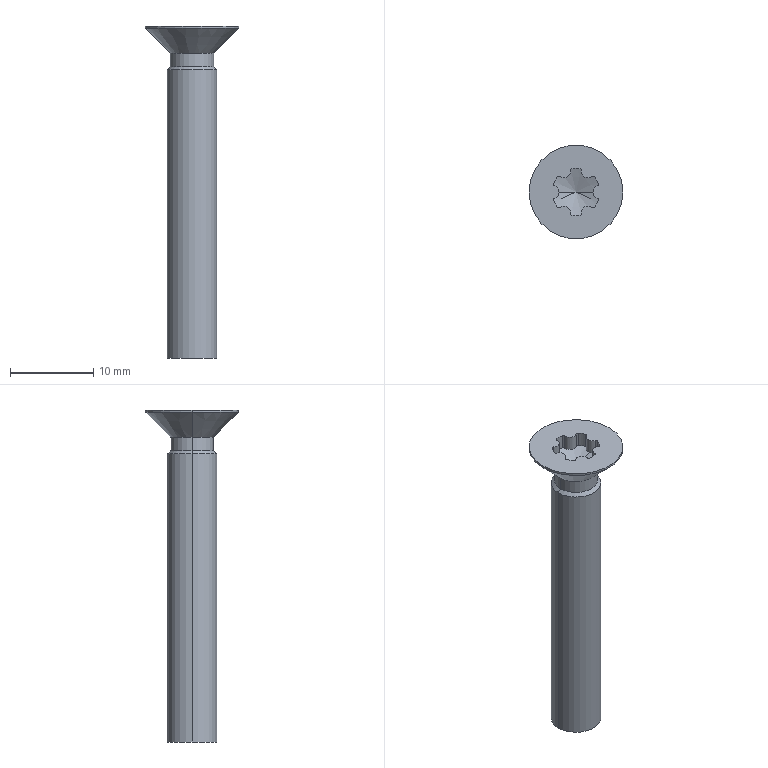Part | SolidWorks | features RevCut 2, Cut 1, Extrusion 1, LPattern 1, Revolution 1 | 1 solid | 51 faces | box 11.3 x 11.3 x 40 mm | volume 1175 mm3 | cylinder 37 | plane 8 | cone 6 | commonest cylinder face diameters 0.4 x16 1.57 x9 5.72 x6 5.196 x2 6 x2 11.3 x2
STEP:
#1=CARTESIAN_POINT('',(0.,0.,37.159));
#2=VERTEX_POINT('',#1);
#3=CARTESIAN_POINT('',(2.86,0.,38.2));
#4=VERTEX_POINT('',#3);
#5=CARTESIAN_POINT('',(2.86,0.,38.2));
#6=DIRECTION('',(0.9397,0.,0.342));
#7=VECTOR('',#6,1000.);
#8=LINE('',#5,#7);
#9=EDGE_CURVE('',#2,#4,#8,.T.);
#10=ORIENTED_EDGE('',*,*,#9,.F.);
#11=CARTESIAN_POINT('',(-2.86,0.,38.2));
#12=VERTEX_POINT('',#11);
#13=CARTESIAN_POINT('',(-2.86,0.,38.2));
#14=DIRECTION('',(-0.9397,0.,0.342));
#15=VECTOR('',#14,1000.);
#16=LINE('',#13,#15);
#17=EDGE_CURVE('',#2,#12,#16,.T.);
#18=ORIENTED_EDGE('',*,*,#17,.T.);
#19=CARTESIAN_POINT('',(-2.685,-0.9847,38.2));
#20=VERTEX_POINT('',#19);
#21=CARTESIAN_POINT('',(0.,0.,38.2));
#22=DIRECTION('',(0.,0.,-1.));
#23=DIRECTION('',(-1.,0.,0.));
#24=AXIS2_PLACEMENT_3D('',#21,#22,#23);
#25=CIRCLE('',#24,2.86);
#26=EDGE_CURVE('',#20,#12,#25,.T.);
#27=ORIENTED_EDGE('',*,*,#26,.F.);
#28=CARTESIAN_POINT('',(-2.195,-1.833,38.2));
#29=VERTEX_POINT('',#28);
#30=CARTESIAN_POINT('',(0.,0.,38.2));
#31=DIRECTION('',(0.,0.,1.));
#32=DIRECTION('',(1.,0.,0.));
#33=AXIS2_PLACEMENT_3D('',#30,#31,#32);
#34=CIRCLE('',#33,2.86);
#35=EDGE_CURVE('',#20,#29,#34,.T.);
#36=ORIENTED_EDGE('',*,*,#35,.T.);
#37=CARTESIAN_POINT('',(-0.4898,-2.818,38.2));
#38=VERTEX_POINT('',#37);
#39=CARTESIAN_POINT('',(0.,0.,38.2));
#40=DIRECTION('',(0.,0.,-1.));
#41=DIRECTION('',(-1.,0.,0.));
#42=AXIS2_PLACEMENT_3D('',#39,#40,#41);
#43=CIRCLE('',#42,2.86);
#44=EDGE_CURVE('',#38,#29,#43,.T.);
#45=ORIENTED_EDGE('',*,*,#44,.F.);
#46=CARTESIAN_POINT('',(0.4898,-2.818,38.2));
#47=VERTEX_POINT('',#46);
#48=CARTESIAN_POINT('',(0.,0.,38.2));
#49=DIRECTION('',(0.,0.,1.));
#50=DIRECTION('',(1.,0.,0.));
#51=AXIS2_PLACEMENT_3D('',#48,#49,#50);
#52=CIRCLE('',#51,2.86);
#53=EDGE_CURVE('',#38,#47,#52,.T.);
#54=ORIENTED_EDGE('',*,*,#53,.T.);
#55=CARTESIAN_POINT('',(2.195,-1.833,38.2));
#56=VERTEX_POINT('',#55);
#57=CARTESIAN_POINT('',(0.,0.,38.2));
#58=DIRECTION('',(0.,0.,-1.));
#59=DIRECTION('',(-1.,0.,0.));
#60=AXIS2_PLACEMENT_3D('',#57,#58,#59);
#61=CIRCLE('',#60,2.86);
#62=EDGE_CURVE('',#56,#47,#61,.T.);
#63=ORIENTED_EDGE('',*,*,#62,.F.);
#64=CARTESIAN_POINT('',(2.685,-0.9847,38.2));
#65=VERTEX_POINT('',#64);
#66=CARTESIAN_POINT('',(0.,0.,38.2));
#67=DIRECTION('',(0.,0.,1.));
#68=DIRECTION('',(1.,0.,0.));
#69=AXIS2_PLACEMENT_3D('',#66,#67,#68);
#70=CIRCLE('',#69,2.86);
#71=EDGE_CURVE('',#56,#65,#70,.T.);
#72=ORIENTED_EDGE('',*,*,#71,.T.);
#73=CARTESIAN_POINT('',(0.,0.,38.2));
#74=DIRECTION('',(0.,0.,-1.));
#75=DIRECTION('',(-1.,0.,0.));
#76=AXIS2_PLACEMENT_3D('',#73,#74,#75);
#77=CIRCLE('',#76,2.86);
#78=EDGE_CURVE('',#4,#65,#77,.T.);
#79=ORIENTED_EDGE('',*,*,#78,.F.);
#80=EDGE_LOOP('',(#10,#18,#27,#36,#45,#54,#63,#72,#79));
#81=FACE_OUTER_BOUND('',#80,.T.);
#82=CARTESIAN_POINT('',(0.,0.,38.2));
#83=DIRECTION('',(0.,0.,1.));
#84=DIRECTION('',(1.,0.,0.));
#85=AXIS2_PLACEMENT_3D('',#82,#83,#84);
#86=CONICAL_SURFACE('',#85,2.86,1.222);
#87=ADVANCED_FACE('',(#81),#86,.F.);
#88=CARTESIAN_POINT('',(-1.918,1.862,38.2));
#89=VERTEX_POINT('',#88);
#90=CARTESIAN_POINT('',(-0.645,2.477,38.2));
#91=VERTEX_POINT('',#90);
#92=CARTESIAN_POINT('',(-1.43,2.477,38.2));
#93=DIRECTION('',(0.,0.,1.));
#94=DIRECTION('',(1.,0.,0.));
#95=AXIS2_PLACEMENT_3D('',#92,#93,#94);
#96=CIRCLE('',#95,0.785);
#97=EDGE_CURVE('',#89,#91,#96,.T.);
#98=ORIENTED_EDGE('',*,*,#97,.T.);
#99=CARTESIAN_POINT('',(-0.645,2.477,40.));
#100=VERTEX_POINT('',#99);
#101=CARTESIAN_POINT('',(-0.645,2.477,38.2));
#102=DIRECTION('',(0.,0.,1.));
#103=VECTOR('',#102,1000.);
#104=LINE('',#101,#103);
#105=EDGE_CURVE('',#91,#100,#104,.T.);
#106=ORIENTED_EDGE('',*,*,#105,.T.);
#107=CARTESIAN_POINT('',(-1.918,1.862,40.));
#108=VERTEX_POINT('',#107);
#109=CARTESIAN_POINT('',(-1.43,2.477,40.));
#110=DIRECTION('',(0.,0.,1.));
#111=DIRECTION('',(1.,0.,0.));
#112=AXIS2_PLACEMENT_3D('',#109,#110,#111);
#113=CIRCLE('',#112,0.785);
#114=EDGE_CURVE('',#108,#100,#113,.T.);
#115=ORIENTED_EDGE('',*,*,#114,.F.);
#116=CARTESIAN_POINT('',(-1.918,1.862,38.2));
#117=DIRECTION('',(0.,0.,1.));
#118=VECTOR('',#117,1000.);
#119=LINE('',#116,#118);
#120=EDGE_CURVE('',#89,#108,#119,.T.);
#121=ORIENTED_EDGE('',*,*,#120,.F.);
#122=EDGE_LOOP('',(#98,#106,#115,#121));
#123=FACE_OUTER_BOUND('',#122,.T.);
#124=CARTESIAN_POINT('',(-1.43,2.477,38.2));
#125=DIRECTION('',(0.,0.,1.));
#126=DIRECTION('',(1.,0.,0.));
#127=AXIS2_PLACEMENT_3D('',#124,#125,#126);
#128=CYLINDRICAL_SURFACE('',#127,0.785);
#129=ADVANCED_FACE('',(#123),#128,.T.);
#130=CARTESIAN_POINT('',(-2.571,-0.7299,38.2));
#131=VERTEX_POINT('',#130);
#132=CARTESIAN_POINT('',(-2.075,0.,38.2));
#133=VERTEX_POINT('',#132);
#134=CARTESIAN_POINT('',(-2.86,0.,38.2));
#135=DIRECTION('',(0.,0.,1.));
#136=DIRECTION('',(1.,0.,0.));
#137=AXIS2_PLACEMENT_3D('',#134,#135,#136);
#138=CIRCLE('',#137,0.785);
#139=EDGE_CURVE('',#131,#133,#138,.T.);
#140=ORIENTED_EDGE('',*,*,#139,.T.);
#141=CARTESIAN_POINT('',(-2.075,0.,40.));
#142=VERTEX_POINT('',#141);
#143=CARTESIAN_POINT('',(-2.075,0.,38.2));
#144=DIRECTION('',(0.,0.,1.));
#145=VECTOR('',#144,1000.);
#146=LINE('',#143,#145);
#147=EDGE_CURVE('',#133,#142,#146,.T.);
#148=ORIENTED_EDGE('',*,*,#147,.T.);
#149=CARTESIAN_POINT('',(-2.571,-0.7299,40.));
#150=VERTEX_POINT('',#149);
#151=CARTESIAN_POINT('',(-2.86,0.,40.));
#152=DIRECTION('',(0.,0.,1.));
#153=DIRECTION('',(1.,0.,0.));
#154=AXIS2_PLACEMENT_3D('',#151,#152,#153);
#155=CIRCLE('',#154,0.785);
#156=EDGE_CURVE('',#150,#142,#155,.T.);
#157=ORIENTED_EDGE('',*,*,#156,.F.);
#158=CARTESIAN_POINT('',(-2.571,-0.7299,38.2));
#159=DIRECTION('',(0.,0.,1.));
#160=VECTOR('',#159,1000.);
#161=LINE('',#158,#160);
#162=EDGE_CURVE('',#131,#150,#161,.T.);
#163=ORIENTED_EDGE('',*,*,#162,.F.);
#164=EDGE_LOOP('',(#140,#148,#157,#163));
#165=FACE_OUTER_BOUND('',#164,.T.);
#166=CARTESIAN_POINT('',(-2.86,0.,38.2));
#167=DIRECTION('',(0.,0.,1.));
#168=DIRECTION('',(1.,0.,0.));
#169=AXIS2_PLACEMENT_3D('',#166,#167,#168);
#170=CYLINDRICAL_SURFACE('',#169,0.785);
#171=ADVANCED_FACE('',(#165),#170,.T.);
#172=CARTESIAN_POINT('',(-0.645,-2.477,38.2));
#173=VERTEX_POINT('',#172);
#174=CARTESIAN_POINT('',(-0.6534,-2.591,38.2));
#175=VERTEX_POINT('',#174);
#176=CARTESIAN_POINT('',(-1.43,-2.477,38.2));
#177=DIRECTION('',(0.,0.,-1.));
#178=DIRECTION('',(-1.,0.,0.));
#179=AXIS2_PLACEMENT_3D('',#176,#177,#178);
#180=CIRCLE('',#179,0.785);
#181=EDGE_CURVE('',#173,#175,#180,.T.);
#182=ORIENTED_EDGE('',*,*,#181,.F.);
#183=CARTESIAN_POINT('',(-0.645,-2.477,40.));
#184=VERTEX_POINT('',#183);
#185=CARTESIAN_POINT('',(-0.645,-2.477,38.2));
#186=DIRECTION('',(0.,0.,1.));
#187=VECTOR('',#186,1000.);
#188=LINE('',#185,#187);
#189=EDGE_CURVE('',#173,#184,#188,.T.);
#190=ORIENTED_EDGE('',*,*,#189,.T.);
#191=CARTESIAN_POINT('',(-0.6534,-2.591,40.));
#192=VERTEX_POINT('',#191);
#193=CARTESIAN_POINT('',(-1.43,-2.477,40.));
#194=DIRECTION('',(0.,0.,-1.));
#195=DIRECTION('',(-1.,0.,0.));
#196=AXIS2_PLACEMENT_3D('',#193,#194,#195);
#197=CIRCLE('',#196,0.785);
#198=EDGE_CURVE('',#184,#192,#197,.T.);
#199=ORIENTED_EDGE('',*,*,#198,.T.);
#200=CARTESIAN_POINT('',(-0.6534,-2.591,38.2));
#201=DIRECTION('',(0.,0.,1.));
#202=VECTOR('',#201,1000.);
#203=LINE('',#200,#202);
#204=EDGE_CURVE('',#175,#192,#203,.T.);
#205=ORIENTED_EDGE('',*,*,#204,.F.);
#206=EDGE_LOOP('',(#182,#190,#199,#205));
#207=FACE_OUTER_BOUND('',#206,.T.);
#208=CARTESIAN_POINT('',(-1.43,-2.477,38.2));
#209=DIRECTION('',(0.,0.,1.));
#210=DIRECTION('',(1.,0.,0.));
#211=AXIS2_PLACEMENT_3D('',#208,#209,#210);
#212=CYLINDRICAL_SURFACE('',#211,0.785);
#213=ADVANCED_FACE('',(#207),#212,.T.);
#214=CARTESIAN_POINT('',(0.6556,-2.621,38.2));
#215=VERTEX_POINT('',#214);
#216=CARTESIAN_POINT('',(0.6534,-2.591,38.2));
#217=VERTEX_POINT('',#216);
#218=CARTESIAN_POINT('',(0.4556,-2.621,38.2));
#219=DIRECTION('',(0.,0.,1.));
#220=DIRECTION('',(1.,0.,0.));
#221=AXIS2_PLACEMENT_3D('',#218,#219,#220);
#222=CIRCLE('',#221,0.2);
#223=EDGE_CURVE('',#215,#217,#222,.T.);
#224=ORIENTED_EDGE('',*,*,#223,.F.);
#225=CARTESIAN_POINT('',(0.6556,-2.621,40.));
#226=VERTEX_POINT('',#225);
#227=CARTESIAN_POINT('',(0.6556,-2.621,38.2));
#228=DIRECTION('',(0.,0.,1.));
#229=VECTOR('',#228,1000.);
#230=LINE('',#227,#229);
#231=EDGE_CURVE('',#215,#226,#230,.T.);
#232=ORIENTED_EDGE('',*,*,#231,.T.);
#233=CARTESIAN_POINT('',(0.6534,-2.591,40.));
#234=VERTEX_POINT('',#233);
#235=CARTESIAN_POINT('',(0.4556,-2.621,40.));
#236=DIRECTION('',(0.,0.,1.));
#237=DIRECTION('',(1.,0.,0.));
#238=AXIS2_PLACEMENT_3D('',#235,#236,#237);
#239=CIRCLE('',#238,0.2);
#240=EDGE_CURVE('',#226,#234,#239,.T.);
#241=ORIENTED_EDGE('',*,*,#240,.T.);
#242=CARTESIAN_POINT('',(0.6534,-2.591,38.2));
#243=DIRECTION('',(0.,0.,1.));
#244=VECTOR('',#243,1000.);
#245=LINE('',#242,#244);
#246=EDGE_CURVE('',#217,#234,#245,.T.);
#247=ORIENTED_EDGE('',*,*,#246,.F.);
#248=EDGE_LOOP('',(#224,#232,#241,#247));
#249=FACE_OUTER_BOUND('',#248,.T.);
#250=CARTESIAN_POINT('',(0.4556,-2.621,38.2));
#251=DIRECTION('',(0.,0.,1.));
#252=DIRECTION('',(1.,0.,0.));
#253=AXIS2_PLACEMENT_3D('',#250,#251,#252);
#254=CYLINDRICAL_SURFACE('',#253,0.2);
#255=ADVANCED_FACE('',(#249),#254,.F.);
#256=CARTESIAN_POINT('',(2.697,-0.9158,38.2));
#257=VERTEX_POINT('',#256);
#258=CARTESIAN_POINT('',(2.571,-0.7299,38.2));
#259=VERTEX_POINT('',#258);
#260=CARTESIAN_POINT('',(2.497,-0.9158,38.2));
#261=DIRECTION('',(0.,0.,1.));
#262=DIRECTION('',(1.,0.,0.));
#263=AXIS2_PLACEMENT_3D('',#260,#261,#262);
#264=CIRCLE('',#263,0.2);
#265=EDGE_CURVE('',#257,#259,#264,.T.);
#266=ORIENTED_EDGE('',*,*,#265,.F.);
#267=CARTESIAN_POINT('',(2.697,-0.9158,40.));
#268=VERTEX_POINT('',#267);
#269=CARTESIAN_POINT('',(2.697,-0.9158,38.2));
#270=DIRECTION('',(0.,0.,1.));
#271=VECTOR('',#270,1000.);
#272=LINE('',#269,#271);
#273=EDGE_CURVE('',#257,#268,#272,.T.);
#274=ORIENTED_EDGE('',*,*,#273,.T.);
#275=CARTESIAN_POINT('',(2.571,-0.7299,40.));
#276=VERTEX_POINT('',#275);
#277=CARTESIAN_POINT('',(2.497,-0.9158,40.));
#278=DIRECTION('',(0.,0.,1.));
#279=DIRECTION('',(1.,0.,0.));
#280=AXIS2_PLACEMENT_3D('',#277,#278,#279);
#281=CIRCLE('',#280,0.2);
#282=EDGE_CURVE('',#268,#276,#281,.T.);
#283=ORIENTED_EDGE('',*,*,#282,.T.);
#284=CARTESIAN_POINT('',(2.571,-0.7299,38.2));
#285=DIRECTION('',(0.,0.,1.));
#286=VECTOR('',#285,1000.);
#287=LINE('',#284,#286);
#288=EDGE_CURVE('',#259,#276,#287,.T.);
#289=ORIENTED_EDGE('',*,*,#288,.F.);
#290=EDGE_LOOP('',(#266,#274,#283,#289));
#291=FACE_OUTER_BOUND('',#290,.T.);
#292=CARTESIAN_POINT('',(2.497,-0.9158,38.2));
#293=DIRECTION('',(0.,0.,1.));
#294=DIRECTION('',(1.,0.,0.));
#295=AXIS2_PLACEMENT_3D('',#292,#293,#294);
#296=CYLINDRICAL_SURFACE('',#295,0.2);
#297=ADVANCED_FACE('',(#291),#296,.F.);
#298=CARTESIAN_POINT('',(2.685,0.9847,38.2));
#299=VERTEX_POINT('',#298);
#300=CARTESIAN_POINT('',(2.697,0.9158,38.2));
#301=VERTEX_POINT('',#300);
#302=CARTESIAN_POINT('',(2.497,0.9158,38.2));
#303=DIRECTION('',(0.,0.,-1.));
#304=DIRECTION('',(-1.,0.,0.));
#305=AXIS2_PLACEMENT_3D('',#302,#303,#304);
#306=CIRCLE('',#305,0.2);
#307=EDGE_CURVE('',#299,#301,#306,.T.);
#308=ORIENTED_EDGE('',*,*,#307,.T.);
#309=CARTESIAN_POINT('',(2.697,0.9158,40.));
#310=VERTEX_POINT('',#309);
#311=CARTESIAN_POINT('',(2.697,0.9158,38.2));
#312=DIRECTION('',(0.,0.,1.));
#313=VECTOR('',#312,1000.);
#314=LINE('',#311,#313);
#315=EDGE_CURVE('',#301,#310,#314,.T.);
#316=ORIENTED_EDGE('',*,*,#315,.T.);
#317=CARTESIAN_POINT('',(2.685,0.9847,40.));
#318=VERTEX_POINT('',#317);
#319=CARTESIAN_POINT('',(2.497,0.9158,40.));
#320=DIRECTION('',(0.,0.,-1.));
#321=DIRECTION('',(-1.,0.,0.));
#322=AXIS2_PLACEMENT_3D('',#319,#320,#321);
#323=CIRCLE('',#322,0.2);
#324=EDGE_CURVE('',#318,#310,#323,.T.);
#325=ORIENTED_EDGE('',*,*,#324,.F.);
#326=CARTESIAN_POINT('',(2.685,0.9847,38.2));
#327=DIRECTION('',(0.,0.,1.));
#328=VECTOR('',#327,1000.);
#329=LINE('',#326,#328);
#330=EDGE_CURVE('',#299,#318,#329,.T.);
#331=ORIENTED_EDGE('',*,*,#330,.F.);
#332=EDGE_LOOP('',(#308,#316,#325,#331));
#333=FACE_OUTER_BOUND('',#332,.T.);
#334=CARTESIAN_POINT('',(2.497,0.9158,38.2));
#335=DIRECTION('',(0.,0.,1.));
#336=DIRECTION('',(1.,0.,0.));
#337=AXIS2_PLACEMENT_3D('',#334,#335,#336);
#338=CYLINDRICAL_SURFACE('',#337,0.2);
#339=ADVANCED_FACE('',(#333),#338,.F.);
#340=CARTESIAN_POINT('',(0.4898,2.818,38.2));
#341=VERTEX_POINT('',#340);
#342=CARTESIAN_POINT('',(0.6556,2.621,38.2));
#343=VERTEX_POINT('',#342);
#344=CARTESIAN_POINT('',(0.4556,2.621,38.2));
#345=DIRECTION('',(0.,0.,-1.));
#346=DIRECTION('',(-1.,0.,0.));
#347=AXIS2_PLACEMENT_3D('',#344,#345,#346);
#348=CIRCLE('',#347,0.2);
#349=EDGE_CURVE('',#341,#343,#348,.T.);
#350=ORIENTED_EDGE('',*,*,#349,.T.);
#351=CARTESIAN_POINT('',(0.6556,2.621,40.));
#352=VERTEX_POINT('',#351);
#353=CARTESIAN_POINT('',(0.6556,2.621,38.2));
#354=DIRECTION('',(0.,0.,1.));
#355=VECTOR('',#354,1000.);
#356=LINE('',#353,#355);
#357=EDGE_CURVE('',#343,#352,#356,.T.);
#358=ORIENTED_EDGE('',*,*,#357,.T.);
#359=CARTESIAN_POINT('',(0.4898,2.818,40.));
#360=VERTEX_POINT('',#359);
#361=CARTESIAN_POINT('',(0.4556,2.621,40.));
#362=DIRECTION('',(0.,0.,-1.));
#363=DIRECTION('',(-1.,0.,0.));
#364=AXIS2_PLACEMENT_3D('',#361,#362,#363);
#365=CIRCLE('',#364,0.2);
#366=EDGE_CURVE('',#360,#352,#365,.T.);
#367=ORIENTED_EDGE('',*,*,#366,.F.);
#368=CARTESIAN_POINT('',(0.4898,2.818,38.2));
#369=DIRECTION('',(0.,0.,1.));
#370=VECTOR('',#369,1000.);
#371=LINE('',#368,#370);
#372=EDGE_CURVE('',#341,#360,#371,.T.);
#373=ORIENTED_EDGE('',*,*,#372,.F.);
#374=EDGE_LOOP('',(#350,#358,#367,#373));
#375=FACE_OUTER_BOUND('',#374,.T.);
#376=CARTESIAN_POINT('',(0.4556,2.621,38.2));
#377=DIRECTION('',(0.,0.,1.));
#378=DIRECTION('',(1.,0.,0.));
#379=AXIS2_PLACEMENT_3D('',#376,#377,#378);
#380=CYLINDRICAL_SURFACE('',#379,0.2);
#381=ADVANCED_FACE('',(#375),#380,.F.);
#382=CARTESIAN_POINT('',(-2.598,0.,35.102));
#383=VERTEX_POINT('',#382);
#384=CARTESIAN_POINT('',(2.598,0.,35.102));
#385=VERTEX_POINT('',#384);
#386=CARTESIAN_POINT('',(0.,0.,35.102));
#387=DIRECTION('',(0.,0.,-1.));
#388=DIRECTION('',(-1.,0.,0.));
#389=AXIS2_PLACEMENT_3D('',#386,#387,#388);
#390=CIRCLE('',#389,2.598);
#391=EDGE_CURVE('',#383,#385,#390,.T.);
#392=ORIENTED_EDGE('',*,*,#391,.T.);
#393=CARTESIAN_POINT('',(3.,0.,34.7));
#394=VERTEX_POINT('',#393);
#395=CARTESIAN_POINT('',(2.598,0.,35.102));
#396=DIRECTION('',(0.7071,0.,-0.7071));
#397=VECTOR('',#396,1000.);
#398=LINE('',#395,#397);
#399=EDGE_CURVE('',#385,#394,#398,.T.);
#400=ORIENTED_EDGE('',*,*,#399,.T.);
#401=CARTESIAN_POINT('',(-3.,0.,34.7));
#402=VERTEX_POINT('',#401);
#403=CARTESIAN_POINT('',(0.,0.,34.7));
#404=DIRECTION('',(0.,0.,1.));
#405=DIRECTION('',(1.,0.,0.));
#406=AXIS2_PLACEMENT_3D('',#403,#404,#405);
#407=CIRCLE('',#406,3.);
#408=EDGE_CURVE('',#394,#402,#407,.T.);
#409=ORIENTED_EDGE('',*,*,#408,.T.);
#410=CARTESIAN_POINT('',(-2.598,0.,35.102));
#411=DIRECTION('',(-0.7071,0.,-0.7071));
#412=VECTOR('',#411,1000.);
#413=LINE('',#410,#412);
#414=EDGE_CURVE('',#383,#402,#413,.T.);
#415=ORIENTED_EDGE('',*,*,#414,.F.);
#416=EDGE_LOOP('',(#392,#400,#409,#415));
#417=FACE_OUTER_BOUND('',#416,.T.);
#418=CARTESIAN_POINT('',(0.,0.,35.102));
#419=DIRECTION('',(0.,0.,-1.));
#420=DIRECTION('',(-1.,0.,0.));
#421=AXIS2_PLACEMENT_3D('',#418,#419,#420);
#422=CONICAL_SURFACE('',#421,2.598,0.7854);
#423=ADVANCED_FACE('',(#417),#422,.T.);
#424=CARTESIAN_POINT('',(-2.598,0.,36.7));
#425=VERTEX_POINT('',#424);
#426=CARTESIAN_POINT('',(2.598,0.,36.7));
#427=VERTEX_POINT('',#426);
#428=CARTESIAN_POINT('',(0.,0.,36.7));
#429=DIRECTION('',(0.,0.,-1.));
#430=DIRECTION('',(-1.,0.,0.));
#431=AXIS2_PLACEMENT_3D('',#428,#429,#430);
#432=CIRCLE('',#431,2.598);
#433=EDGE_CURVE('',#425,#427,#432,.T.);
#434=ORIENTED_EDGE('',*,*,#433,.T.);
#435=CARTESIAN_POINT('',(2.598,0.,-0.3936));
#436=DIRECTION('',(0.,0.,-1.));
#437=VECTOR('',#436,1000.);
#438=LINE('',#435,#437);
#439=EDGE_CURVE('',#427,#385,#438,.T.);
#440=ORIENTED_EDGE('',*,*,#439,.T.);
#441=ORIENTED_EDGE('',*,*,#391,.F.);
#442=CARTESIAN_POINT('',(-2.598,0.,-0.3936));
#443=DIRECTION('',(0.,0.,-1.));
#444=VECTOR('',#443,1000.);
#445=LINE('',#442,#444);
#446=EDGE_CURVE('',#425,#383,#445,.T.);
#447=ORIENTED_EDGE('',*,*,#446,.F.);
#448=EDGE_LOOP('',(#434,#440,#441,#447));
#449=FACE_OUTER_BOUND('',#448,.T.);
#450=CARTESIAN_POINT('',(0.,0.,-0.3936));
#451=DIRECTION('',(0.,0.,-1.));
#452=DIRECTION('',(-1.,0.,0.));
#453=AXIS2_PLACEMENT_3D('',#450,#451,#452);
#454=CYLINDRICAL_SURFACE('',#453,2.598);
#455=ADVANCED_FACE('',(#449),#454,.T.);
#456=ORIENTED_EDGE('',*,*,#433,.F.);
#457=CARTESIAN_POINT('',(-5.65,0.,39.752));
#458=VERTEX_POINT('',#457);
#459=CARTESIAN_POINT('',(-2.598,0.,36.7));
#460=DIRECTION('',(-0.7071,0.,0.7071));
#461=VECTOR('',#460,1000.);
#462=LINE('',#459,#461);
#463=EDGE_CURVE('',#425,#458,#462,.T.);
#464=ORIENTED_EDGE('',*,*,#463,.T.);
#465=CARTESIAN_POINT('',(5.65,0.,39.752));
#466=VERTEX_POINT('',#465);
#467=CARTESIAN_POINT('',(0.,0.,39.752));
#468=DIRECTION('',(0.,0.,-1.));
#469=DIRECTION('',(-1.,0.,0.));
#470=AXIS2_PLACEMENT_3D('',#467,#468,#469);
#471=CIRCLE('',#470,5.65);
#472=EDGE_CURVE('',#458,#466,#471,.T.);
#473=ORIENTED_EDGE('',*,*,#472,.T.);
#474=CARTESIAN_POINT('',(2.598,0.,36.7));
#475=DIRECTION('',(0.7071,0.,0.7071));
#476=VECTOR('',#475,1000.);
#477=LINE('',#474,#476);
#478=EDGE_CURVE('',#427,#466,#477,.T.);
#479=ORIENTED_EDGE('',*,*,#478,.F.);
#480=EDGE_LOOP('',(#456,#464,#473,#479));
#481=FACE_OUTER_BOUND('',#480,.T.);
#482=CARTESIAN_POINT('',(0.,0.,36.7));
#483=DIRECTION('',(0.,0.,1.));
#484=DIRECTION('',(1.,0.,0.));
#485=AXIS2_PLACEMENT_3D('',#482,#483,#484);
#486=CONICAL_SURFACE('',#485,2.598,0.7854);
#487=ADVANCED_FACE('',(#481),#486,.T.);
#488=CARTESIAN_POINT('',(-5.65,0.,40.));
#489=VERTEX_POINT('',#488);
#490=CARTESIAN_POINT('',(5.65,0.,40.));
#491=VERTEX_POINT('',#490);
#492=CARTESIAN_POINT('',(0.,0.,40.));
#493=DIRECTION('',(0.,0.,-1.));
#494=DIRECTION('',(-1.,0.,0.));
#495=AXIS2_PLACEMENT_3D('',#492,#493,#494);
#496=CIRCLE('',#495,5.65);
#497=EDGE_CURVE('',#489,#491,#496,.T.);
#498=ORIENTED_EDGE('',*,*,#497,.T.);
#499=CARTESIAN_POINT('',(5.65,0.,-0.3936));
#500=DIRECTION('',(0.,0.,-1.));
#501=VECTOR('',#500,1000.);
#502=LINE('',#499,#501);
#503=EDGE_CURVE('',#491,#466,#502,.T.);
#504=ORIENTED_EDGE('',*,*,#503,.T.);
#505=ORIENTED_EDGE('',*,*,#472,.F.);
#506=CARTESIAN_POINT('',(-5.65,0.,-0.3936));
#507=DIRECTION('',(0.,0.,-1.));
#508=VECTOR('',#507,1000.);
#509=LINE('',#506,#508);
#510=EDGE_CURVE('',#489,#458,#509,.T.);
#511=ORIENTED_EDGE('',*,*,#510,.F.);
#512=EDGE_LOOP('',(#498,#504,#505,#511));
#513=FACE_OUTER_BOUND('',#512,.T.);
#514=CARTESIAN_POINT('',(0.,0.,-0.3936));
#515=DIRECTION('',(0.,0.,-1.));
#516=DIRECTION('',(-1.,0.,0.));
#517=AXIS2_PLACEMENT_3D('',#514,#515,#516);
#518=CYLINDRICAL_SURFACE('',#517,5.65);
#519=ADVANCED_FACE('',(#513),#518,.T.);
#520=ORIENTED_EDGE('',*,*,#408,.F.);
#521=CARTESIAN_POINT('',(3.,0.,0.));
#522=VERTEX_POINT('',#521);
#523=CARTESIAN_POINT('',(3.,0.,34.7));
#524=DIRECTION('',(0.,0.,-1.));
#525=VECTOR('',#524,1000.);
#526=LINE('',#523,#525);
#527=EDGE_CURVE('',#394,#522,#526,.T.);
#528=ORIENTED_EDGE('',*,*,#527,.T.);
#529=CARTESIAN_POINT('',(-3.,0.,0.));
#530=VERTEX_POINT('',#529);
#531=CARTESIAN_POINT('',(0.,0.,0.));
#532=DIRECTION('',(0.,0.,1.));
#533=DIRECTION('',(1.,0.,0.));
#534=AXIS2_PLACEMENT_3D('',#531,#532,#533);
#535=CIRCLE('',#534,3.);
#536=EDGE_CURVE('',#522,#530,#535,.T.);
#537=ORIENTED_EDGE('',*,*,#536,.T.);
#538=CARTESIAN_POINT('',(-3.,0.,34.7));
#539=DIRECTION('',(0.,0.,-1.));
#540=VECTOR('',#539,1000.);
#541=LINE('',#538,#540);
#542=EDGE_CURVE('',#402,#530,#541,.T.);
#543=ORIENTED_EDGE('',*,*,#542,.F.);
#544=EDGE_LOOP('',(#520,#528,#537,#543));
#545=FACE_OUTER_BOUND('',#544,.T.);
#546=CARTESIAN_POINT('',(0.,0.,34.7));
#547=DIRECTION('',(0.,0.,-1.));
#548=DIRECTION('',(-1.,0.,0.));
#549=AXIS2_PLACEMENT_3D('',#546,#547,#548);
#550=CYLINDRICAL_SURFACE('',#549,3.);
#551=ADVANCED_FACE('',(#545),#550,.T.);
#552=ORIENTED_EDGE('',*,*,#497,.F.);
#553=CARTESIAN_POINT('',(0.,0.,40.));
#554=DIRECTION('',(0.,0.,-1.));
#555=DIRECTION('',(-1.,0.,0.));
#556=AXIS2_PLACEMENT_3D('',#553,#554,#555);
#557=CIRCLE('',#556,5.65);
#558=EDGE_CURVE('',#491,#489,#557,.T.);
#559=ORIENTED_EDGE('',*,*,#558,.F.);
#560=EDGE_LOOP('',(#552,#559));
#561=FACE_OUTER_BOUND('',#560,.T.);
#562=CARTESIAN_POINT('',(-0.4898,2.818,40.));
#563=VERTEX_POINT('',#562);
#564=CARTESIAN_POINT('',(0.,0.,40.));
#565=DIRECTION('',(0.,0.,1.));
#566=DIRECTION('',(1.,0.,0.));
#567=AXIS2_PLACEMENT_3D('',#564,#565,#566);
#568=CIRCLE('',#567,2.86);
#569=EDGE_CURVE('',#360,#563,#568,.T.);
#570=ORIENTED_EDGE('',*,*,#569,.F.);
#571=ORIENTED_EDGE('',*,*,#366,.T.);
#572=CARTESIAN_POINT('',(0.6534,2.591,40.));
#573=VERTEX_POINT('',#572);
#574=CARTESIAN_POINT('',(0.4556,2.621,40.));
#575=DIRECTION('',(0.,0.,-1.));
#576=DIRECTION('',(-1.,0.,0.));
#577=AXIS2_PLACEMENT_3D('',#574,#575,#576);
#578=CIRCLE('',#577,0.2);
#579=EDGE_CURVE('',#352,#573,#578,.T.);
#580=ORIENTED_EDGE('',*,*,#579,.T.);
#581=CARTESIAN_POINT('',(1.918,1.862,40.));
#582=VERTEX_POINT('',#581);
#583=CARTESIAN_POINT('',(1.43,2.477,40.));
#584=DIRECTION('',(0.,0.,-1.));
#585=DIRECTION('',(-1.,0.,0.));
#586=AXIS2_PLACEMENT_3D('',#583,#584,#585);
#587=CIRCLE('',#586,0.785);
#588=EDGE_CURVE('',#582,#573,#587,.T.);
#589=ORIENTED_EDGE('',*,*,#588,.F.);
#590=CARTESIAN_POINT('',(2.195,1.833,40.));
#591=VERTEX_POINT('',#590);
#592=CARTESIAN_POINT('',(2.042,1.705,40.));
#593=DIRECTION('',(0.,0.,1.));
#594=DIRECTION('',(1.,0.,0.));
#595=AXIS2_PLACEMENT_3D('',#592,#593,#594);
#596=CIRCLE('',#595,0.2);
#597=EDGE_CURVE('',#591,#582,#596,.T.);
#598=ORIENTED_EDGE('',*,*,#597,.F.);
#599=CARTESIAN_POINT('',(0.,0.,40.));
#600=DIRECTION('',(0.,0.,1.));
#601=DIRECTION('',(1.,0.,0.));
#602=AXIS2_PLACEMENT_3D('',#599,#600,#601);
#603=CIRCLE('',#602,2.86);
#604=EDGE_CURVE('',#318,#591,#603,.T.);
#605=ORIENTED_EDGE('',*,*,#604,.F.);
#606=ORIENTED_EDGE('',*,*,#324,.T.);
#607=CARTESIAN_POINT('',(2.571,0.7299,40.));
#608=VERTEX_POINT('',#607);
#609=CARTESIAN_POINT('',(2.497,0.9158,40.));
#610=DIRECTION('',(0.,0.,-1.));
#611=DIRECTION('',(-1.,0.,0.));
#612=AXIS2_PLACEMENT_3D('',#609,#610,#611);
#613=CIRCLE('',#612,0.2);
#614=EDGE_CURVE('',#310,#608,#613,.T.);
#615=ORIENTED_EDGE('',*,*,#614,.T.);
#616=CARTESIAN_POINT('',(2.86,0.,40.));
#617=DIRECTION('',(0.,0.,-1.));
#618=DIRECTION('',(-1.,0.,0.));
#619=AXIS2_PLACEMENT_3D('',#616,#617,#618);
#620=CIRCLE('',#619,0.785);
#621=EDGE_CURVE('',#276,#608,#620,.T.);
#622=ORIENTED_EDGE('',*,*,#621,.F.);
#623=ORIENTED_EDGE('',*,*,#282,.F.);
#624=CARTESIAN_POINT('',(2.685,-0.9847,40.));
#625=VERTEX_POINT('',#624);
#626=CARTESIAN_POINT('',(2.497,-0.9158,40.));
#627=DIRECTION('',(0.,0.,1.));
#628=DIRECTION('',(1.,0.,0.));
#629=AXIS2_PLACEMENT_3D('',#626,#627,#628);
#630=CIRCLE('',#629,0.2);
#631=EDGE_CURVE('',#625,#268,#630,.T.);
#632=ORIENTED_EDGE('',*,*,#631,.F.);
#633=CARTESIAN_POINT('',(2.195,-1.833,40.));
#634=VERTEX_POINT('',#633);
#635=CARTESIAN_POINT('',(0.,0.,40.));
#636=DIRECTION('',(0.,0.,1.));
#637=DIRECTION('',(1.,0.,0.));
#638=AXIS2_PLACEMENT_3D('',#635,#636,#637);
#639=CIRCLE('',#638,2.86);
#640=EDGE_CURVE('',#634,#625,#639,.T.);
#641=ORIENTED_EDGE('',*,*,#640,.F.);
#642=CARTESIAN_POINT('',(1.918,-1.862,40.));
#643=VERTEX_POINT('',#642);
#644=CARTESIAN_POINT('',(2.042,-1.705,40.));
#645=DIRECTION('',(0.,0.,-1.));
#646=DIRECTION('',(-1.,0.,0.));
#647=AXIS2_PLACEMENT_3D('',#644,#645,#646);
#648=CIRCLE('',#647,0.2);
#649=EDGE_CURVE('',#634,#643,#648,.T.);
#650=ORIENTED_EDGE('',*,*,#649,.T.);
#651=CARTESIAN_POINT('',(1.43,-2.477,40.));
#652=DIRECTION('',(0.,0.,1.));
#653=DIRECTION('',(1.,0.,0.));
#654=AXIS2_PLACEMENT_3D('',#651,#652,#653);
#655=CIRCLE('',#654,0.785);
#656=EDGE_CURVE('',#643,#234,#655,.T.);
#657=ORIENTED_EDGE('',*,*,#656,.T.);
#658=ORIENTED_EDGE('',*,*,#240,.F.);
#659=CARTESIAN_POINT('',(0.4898,-2.818,40.));
#660=VERTEX_POINT('',#659);
#661=CARTESIAN_POINT('',(0.4556,-2.621,40.));
#662=DIRECTION('',(0.,0.,1.));
#663=DIRECTION('',(1.,0.,0.));
#664=AXIS2_PLACEMENT_3D('',#661,#662,#663);
#665=CIRCLE('',#664,0.2);
#666=EDGE_CURVE('',#660,#226,#665,.T.);
#667=ORIENTED_EDGE('',*,*,#666,.F.);
#668=CARTESIAN_POINT('',(-0.4898,-2.818,40.));
#669=VERTEX_POINT('',#668);
#670=CARTESIAN_POINT('',(0.,0.,40.));
#671=DIRECTION('',(0.,0.,1.));
#672=DIRECTION('',(1.,0.,0.));
#673=AXIS2_PLACEMENT_3D('',#670,#671,#672);
#674=CIRCLE('',#673,2.86);
#675=EDGE_CURVE('',#669,#660,#674,.T.);
#676=ORIENTED_EDGE('',*,*,#675,.F.);
#677=CARTESIAN_POINT('',(-0.4556,-2.621,40.));
#678=DIRECTION('',(0.,0.,-1.));
#679=DIRECTION('',(-1.,0.,0.));
#680=AXIS2_PLACEMENT_3D('',#677,#678,#679);
#681=CIRCLE('',#680,0.2);
#682=EDGE_CURVE('',#669,#192,#681,.T.);
#683=ORIENTED_EDGE('',*,*,#682,.T.);
#684=ORIENTED_EDGE('',*,*,#198,.F.);
#685=CARTESIAN_POINT('',(-1.918,-1.862,40.));
#686=VERTEX_POINT('',#685);
#687=CARTESIAN_POINT('',(-1.43,-2.477,40.));
#688=DIRECTION('',(0.,0.,-1.));
#689=DIRECTION('',(-1.,0.,0.));
#690=AXIS2_PLACEMENT_3D('',#687,#688,#689);
#691=CIRCLE('',#690,0.785);
#692=EDGE_CURVE('',#686,#184,#691,.T.);
#693=ORIENTED_EDGE('',*,*,#692,.F.);
#694=CARTESIAN_POINT('',(-2.195,-1.833,40.));
#695=VERTEX_POINT('',#694);
#696=CARTESIAN_POINT('',(-2.042,-1.705,40.));
#697=DIRECTION('',(0.,0.,1.));
#698=DIRECTION('',(1.,0.,0.));
#699=AXIS2_PLACEMENT_3D('',#696,#697,#698);
#700=CIRCLE('',#699,0.2);
#701=EDGE_CURVE('',#695,#686,#700,.T.);
#702=ORIENTED_EDGE('',*,*,#701,.F.);
#703=CARTESIAN_POINT('',(-2.685,-0.9847,40.));
#704=VERTEX_POINT('',#703);
#705=CARTESIAN_POINT('',(0.,0.,40.));
#706=DIRECTION('',(0.,0.,1.));
#707=DIRECTION('',(1.,0.,0.));
#708=AXIS2_PLACEMENT_3D('',#705,#706,#707);
#709=CIRCLE('',#708,2.86);
#710=EDGE_CURVE('',#704,#695,#709,.T.);
#711=ORIENTED_EDGE('',*,*,#710,.F.);
#712=CARTESIAN_POINT('',(-2.497,-0.9158,40.));
#713=DIRECTION('',(0.,0.,-1.));
#714=DIRECTION('',(-1.,0.,0.));
#715=AXIS2_PLACEMENT_3D('',#712,#713,#714);
#716=CIRCLE('',#715,0.2);
#717=EDGE_CURVE('',#704,#150,#716,.T.);
#718=ORIENTED_EDGE('',*,*,#717,.T.);
#719=ORIENTED_EDGE('',*,*,#156,.T.);
#720=CARTESIAN_POINT('',(-2.571,0.7299,40.));
#721=VERTEX_POINT('',#720);
#722=CARTESIAN_POINT('',(-2.86,0.,40.));
#723=DIRECTION('',(0.,0.,1.));
#724=DIRECTION('',(1.,0.,0.));
#725=AXIS2_PLACEMENT_3D('',#722,#723,#724);
#726=CIRCLE('',#725,0.785);
#727=EDGE_CURVE('',#142,#721,#726,.T.);
#728=ORIENTED_EDGE('',*,*,#727,.T.);
#729=CARTESIAN_POINT('',(-2.685,0.9847,40.));
#730=VERTEX_POINT('',#729);
#731=CARTESIAN_POINT('',(-2.497,0.9158,40.));
#732=DIRECTION('',(0.,0.,1.));
#733=DIRECTION('',(1.,0.,0.));
#734=AXIS2_PLACEMENT_3D('',#731,#732,#733);
#735=CIRCLE('',#734,0.2);
#736=EDGE_CURVE('',#730,#721,#735,.T.);
#737=ORIENTED_EDGE('',*,*,#736,.F.);
#738=CARTESIAN_POINT('',(-2.195,1.833,40.));
#739=VERTEX_POINT('',#738);
#740=CARTESIAN_POINT('',(0.,0.,40.));
#741=DIRECTION('',(0.,0.,1.));
#742=DIRECTION('',(1.,0.,0.));
#743=AXIS2_PLACEMENT_3D('',#740,#741,#742);
#744=CIRCLE('',#743,2.86);
#745=EDGE_CURVE('',#739,#730,#744,.T.);
#746=ORIENTED_EDGE('',*,*,#745,.F.);
#747=CARTESIAN_POINT('',(-2.042,1.705,40.));
#748=DIRECTION('',(0.,0.,-1.));
#749=DIRECTION('',(-1.,0.,0.));
#750=AXIS2_PLACEMENT_3D('',#747,#748,#749);
#751=CIRCLE('',#750,0.2);
#752=EDGE_CURVE('',#739,#108,#751,.T.);
#753=ORIENTED_EDGE('',*,*,#752,.T.);
#754=ORIENTED_EDGE('',*,*,#114,.T.);
#755=CARTESIAN_POINT('',(-0.6534,2.591,40.));
#756=VERTEX_POINT('',#755);
#757=CARTESIAN_POINT('',(-1.43,2.477,40.));
#758=DIRECTION('',(0.,0.,1.));
#759=DIRECTION('',(1.,0.,0.));
#760=AXIS2_PLACEMENT_3D('',#757,#758,#759);
#761=CIRCLE('',#760,0.785);
#762=EDGE_CURVE('',#100,#756,#761,.T.);
#763=ORIENTED_EDGE('',*,*,#762,.T.);
#764=CARTESIAN_POINT('',(-0.4556,2.621,40.));
#765=DIRECTION('',(0.,0.,1.));
#766=DIRECTION('',(1.,0.,0.));
#767=AXIS2_PLACEMENT_3D('',#764,#765,#766);
#768=CIRCLE('',#767,0.2);
#769=EDGE_CURVE('',#563,#756,#768,.T.);
#770=ORIENTED_EDGE('',*,*,#769,.F.);
#771=EDGE_LOOP('',(#570,#571,#580,#589,#598,#605,#606,#615,#622,#623,#632,#641,#650,#657,#658,#667,#676,#683,#684,#693,#702,#711,#718,#719,#728,#737,#746,#753,#754,#763,#770));
#772=FACE_BOUND('',#771,.T.);
#773=CARTESIAN_POINT('',(5.65,0.,40.));
#774=DIRECTION('',(0.,0.,1.));
#775=DIRECTION('',(1.,0.,0.));
#776=AXIS2_PLACEMENT_3D('',#773,#774,#775);
#777=PLANE('',#776);
#778=ADVANCED_FACE('',(#561,#772),#777,.T.);
#779=ORIENTED_EDGE('',*,*,#527,.F.);
#780=CARTESIAN_POINT('',(0.,0.,34.7));
#781=DIRECTION('',(0.,0.,1.));
#782=DIRECTION('',(1.,0.,0.));
#783=AXIS2_PLACEMENT_3D('',#780,#781,#782);
#784=CIRCLE('',#783,3.);
#785=EDGE_CURVE('',#402,#394,#784,.T.);
#786=ORIENTED_EDGE('',*,*,#785,.F.);
#787=ORIENTED_EDGE('',*,*,#542,.T.);
#788=CARTESIAN_POINT('',(0.,0.,0.));
#789=DIRECTION('',(0.,0.,1.));
#790=DIRECTION('',(1.,0.,0.));
#791=AXIS2_PLACEMENT_3D('',#788,#789,#790);
#792=CIRCLE('',#791,3.);
#793=EDGE_CURVE('',#530,#522,#792,.T.);
#794=ORIENTED_EDGE('',*,*,#793,.T.);
#795=EDGE_LOOP('',(#779,#786,#787,#794));
#796=FACE_OUTER_BOUND('',#795,.T.);
#797=CARTESIAN_POINT('',(0.,0.,34.7));
#798=DIRECTION('',(0.,0.,-1.));
#799=DIRECTION('',(-1.,0.,0.));
#800=AXIS2_PLACEMENT_3D('',#797,#798,#799);
#801=CYLINDRICAL_SURFACE('',#800,3.);
#802=ADVANCED_FACE('',(#796),#801,.T.);
#803=ORIENTED_EDGE('',*,*,#793,.F.);
#804=ORIENTED_EDGE('',*,*,#536,.F.);
#805=EDGE_LOOP('',(#803,#804));
#806=FACE_OUTER_BOUND('',#805,.T.);
#807=CARTESIAN_POINT('',(0.,0.,0.));
#808=DIRECTION('',(0.,0.,1.));
#809=DIRECTION('',(1.,0.,0.));
#810=AXIS2_PLACEMENT_3D('',#807,#808,#809);
#811=PLANE('',#810);
#812=ADVANCED_FACE('',(#806),#811,.F.);
#813=ORIENTED_EDGE('',*,*,#503,.F.);
#814=ORIENTED_EDGE('',*,*,#558,.T.);
#815=ORIENTED_EDGE('',*,*,#510,.T.);
#816=CARTESIAN_POINT('',(0.,0.,39.752));
#817=DIRECTION('',(0.,0.,-1.));
#818=DIRECTION('',(-1.,0.,0.));
#819=AXIS2_PLACEMENT_3D('',#816,#817,#818);
#820=CIRCLE('',#819,5.65);
#821=EDGE_CURVE('',#466,#458,#820,.T.);
#822=ORIENTED_EDGE('',*,*,#821,.F.);
#823=EDGE_LOOP('',(#813,#814,#815,#822));
#824=FACE_OUTER_BOUND('',#823,.T.);
#825=CARTESIAN_POINT('',(0.,0.,-0.3936));
#826=DIRECTION('',(0.,0.,-1.));
#827=DIRECTION('',(-1.,0.,0.));
#828=AXIS2_PLACEMENT_3D('',#825,#826,#827);
#829=CYLINDRICAL_SURFACE('',#828,5.65);
#830=ADVANCED_FACE('',(#824),#829,.T.);
#831=ORIENTED_EDGE('',*,*,#463,.F.);
#832=CARTESIAN_POINT('',(0.,0.,36.7));
#833=DIRECTION('',(0.,0.,-1.));
#834=DIRECTION('',(-1.,0.,0.));
#835=AXIS2_PLACEMENT_3D('',#832,#833,#834);
#836=CIRCLE('',#835,2.598);
#837=EDGE_CURVE('',#427,#425,#836,.T.);
#838=ORIENTED_EDGE('',*,*,#837,.F.);
#839=ORIENTED_EDGE('',*,*,#478,.T.);
#840=ORIENTED_EDGE('',*,*,#821,.T.);
#841=EDGE_LOOP('',(#831,#838,#839,#840));
#842=FACE_OUTER_BOUND('',#841,.T.);
#843=CARTESIAN_POINT('',(0.,0.,36.7));
#844=DIRECTION('',(0.,0.,1.));
#845=DIRECTION('',(1.,0.,0.));
#846=AXIS2_PLACEMENT_3D('',#843,#844,#845);
#847=CONICAL_SURFACE('',#846,2.598,0.7854);
#848=ADVANCED_FACE('',(#842),#847,.T.);
#849=ORIENTED_EDGE('',*,*,#439,.F.);
#850=ORIENTED_EDGE('',*,*,#837,.T.);
#851=ORIENTED_EDGE('',*,*,#446,.T.);
#852=CARTESIAN_POINT('',(0.,0.,35.102));
#853=DIRECTION('',(0.,0.,-1.));
#854=DIRECTION('',(-1.,0.,0.));
#855=AXIS2_PLACEMENT_3D('',#852,#853,#854);
#856=CIRCLE('',#855,2.598);
#857=EDGE_CURVE('',#385,#383,#856,.T.);
#858=ORIENTED_EDGE('',*,*,#857,.F.);
#859=EDGE_LOOP('',(#849,#850,#851,#858));
#860=FACE_OUTER_BOUND('',#859,.T.);
#861=CARTESIAN_POINT('',(0.,0.,-0.3936));
#862=DIRECTION('',(0.,0.,-1.));
#863=DIRECTION('',(-1.,0.,0.));
#864=AXIS2_PLACEMENT_3D('',#861,#862,#863);
#865=CYLINDRICAL_SURFACE('',#864,2.598);
#866=ADVANCED_FACE('',(#860),#865,.T.);
#867=ORIENTED_EDGE('',*,*,#399,.F.);
#868=ORIENTED_EDGE('',*,*,#857,.T.);
#869=ORIENTED_EDGE('',*,*,#414,.T.);
#870=ORIENTED_EDGE('',*,*,#785,.T.);
#871=EDGE_LOOP('',(#867,#868,#869,#870));
#872=FACE_OUTER_BOUND('',#871,.T.);
#873=CARTESIAN_POINT('',(0.,0.,35.102));
#874=DIRECTION('',(0.,0.,-1.));
#875=DIRECTION('',(-1.,0.,0.));
#876=AXIS2_PLACEMENT_3D('',#873,#874,#875);
#877=CONICAL_SURFACE('',#876,2.598,0.7854);
#878=ADVANCED_FACE('',(#872),#877,.T.);
#879=ORIENTED_EDGE('',*,*,#357,.F.);
#880=CARTESIAN_POINT('',(0.6534,2.591,38.2));
#881=VERTEX_POINT('',#880);
#882=CARTESIAN_POINT('',(0.4556,2.621,38.2));
#883=DIRECTION('',(0.,0.,-1.));
#884=DIRECTION('',(-1.,0.,0.));
#885=AXIS2_PLACEMENT_3D('',#882,#883,#884);
#886=CIRCLE('',#885,0.2);
#887=EDGE_CURVE('',#343,#881,#886,.T.);
#888=ORIENTED_EDGE('',*,*,#887,.T.);
#889=CARTESIAN_POINT('',(0.6534,2.591,38.2));
#890=DIRECTION('',(0.,0.,1.));
#891=VECTOR('',#890,1000.);
#892=LINE('',#889,#891);
#893=EDGE_CURVE('',#881,#573,#892,.T.);
#894=ORIENTED_EDGE('',*,*,#893,.T.);
#895=ORIENTED_EDGE('',*,*,#579,.F.);
#896=EDGE_LOOP('',(#879,#888,#894,#895));
#897=FACE_OUTER_BOUND('',#896,.T.);
#898=CARTESIAN_POINT('',(0.4556,2.621,38.2));
#899=DIRECTION('',(0.,0.,1.));
#900=DIRECTION('',(1.,0.,0.));
#901=AXIS2_PLACEMENT_3D('',#898,#899,#900);
#902=CYLINDRICAL_SURFACE('',#901,0.2);
#903=ADVANCED_FACE('',(#897),#902,.F.);
#904=ORIENTED_EDGE('',*,*,#588,.T.);
#905=ORIENTED_EDGE('',*,*,#893,.F.);
#906=CARTESIAN_POINT('',(1.918,1.862,38.2));
#907=VERTEX_POINT('',#906);
#908=CARTESIAN_POINT('',(1.43,2.477,38.2));
#909=DIRECTION('',(0.,0.,-1.));
#910=DIRECTION('',(-1.,0.,0.));
#911=AXIS2_PLACEMENT_3D('',#908,#909,#910);
#912=CIRCLE('',#911,0.785);
#913=EDGE_CURVE('',#907,#881,#912,.T.);
#914=ORIENTED_EDGE('',*,*,#913,.F.);
#915=CARTESIAN_POINT('',(1.918,1.862,38.2));
#916=DIRECTION('',(0.,0.,1.));
#917=VECTOR('',#916,1000.);
#918=LINE('',#915,#917);
#919=EDGE_CURVE('',#907,#582,#918,.T.);
#920=ORIENTED_EDGE('',*,*,#919,.T.);
#921=EDGE_LOOP('',(#904,#905,#914,#920));
#922=FACE_OUTER_BOUND('',#921,.T.);
#923=CARTESIAN_POINT('',(1.43,2.477,38.2));
#924=DIRECTION('',(0.,0.,1.));
#925=DIRECTION('',(1.,0.,0.));
#926=AXIS2_PLACEMENT_3D('',#923,#924,#925);
#927=CYLINDRICAL_SURFACE('',#926,0.785);
#928=ADVANCED_FACE('',(#922),#927,.T.);
#929=ORIENTED_EDGE('',*,*,#597,.T.);
#930=ORIENTED_EDGE('',*,*,#919,.F.);
#931=CARTESIAN_POINT('',(2.195,1.833,38.2));
#932=VERTEX_POINT('',#931);
#933=CARTESIAN_POINT('',(2.042,1.705,38.2));
#934=DIRECTION('',(0.,0.,1.));
#935=DIRECTION('',(1.,0.,0.));
#936=AXIS2_PLACEMENT_3D('',#933,#934,#935);
#937=CIRCLE('',#936,0.2);
#938=EDGE_CURVE('',#932,#907,#937,.T.);
#939=ORIENTED_EDGE('',*,*,#938,.F.);
#940=CARTESIAN_POINT('',(2.195,1.833,38.2));
#941=DIRECTION('',(0.,0.,1.));
#942=VECTOR('',#941,1000.);
#943=LINE('',#940,#942);
#944=EDGE_CURVE('',#932,#591,#943,.T.);
#945=ORIENTED_EDGE('',*,*,#944,.T.);
#946=EDGE_LOOP('',(#929,#930,#939,#945));
#947=FACE_OUTER_BOUND('',#946,.T.);
#948=CARTESIAN_POINT('',(2.042,1.705,38.2));
#949=DIRECTION('',(0.,0.,1.));
#950=DIRECTION('',(1.,0.,0.));
#951=AXIS2_PLACEMENT_3D('',#948,#949,#950);
#952=CYLINDRICAL_SURFACE('',#951,0.2);
#953=ADVANCED_FACE('',(#947),#952,.F.);
#954=ORIENTED_EDGE('',*,*,#604,.T.);
#955=ORIENTED_EDGE('',*,*,#944,.F.);
#956=CARTESIAN_POINT('',(0.,0.,38.2));
#957=DIRECTION('',(0.,0.,1.));
#958=DIRECTION('',(1.,0.,0.));
#959=AXIS2_PLACEMENT_3D('',#956,#957,#958);
#960=CIRCLE('',#959,2.86);
#961=EDGE_CURVE('',#299,#932,#960,.T.);
#962=ORIENTED_EDGE('',*,*,#961,.F.);
#963=ORIENTED_EDGE('',*,*,#330,.T.);
#964=EDGE_LOOP('',(#954,#955,#962,#963));
#965=FACE_OUTER_BOUND('',#964,.T.);
#966=CARTESIAN_POINT('',(0.,0.,38.2));
#967=DIRECTION('',(0.,0.,1.));
#968=DIRECTION('',(1.,0.,0.));
#969=AXIS2_PLACEMENT_3D('',#966,#967,#968);
#970=CYLINDRICAL_SURFACE('',#969,2.86);
#971=ADVANCED_FACE('',(#965),#970,.F.);
#972=ORIENTED_EDGE('',*,*,#315,.F.);
#973=CARTESIAN_POINT('',(2.571,0.7299,38.2));
#974=VERTEX_POINT('',#973);
#975=CARTESIAN_POINT('',(2.497,0.9158,38.2));
#976=DIRECTION('',(0.,0.,-1.));
#977=DIRECTION('',(-1.,0.,0.));
#978=AXIS2_PLACEMENT_3D('',#975,#976,#977);
#979=CIRCLE('',#978,0.2);
#980=EDGE_CURVE('',#301,#974,#979,.T.);
#981=ORIENTED_EDGE('',*,*,#980,.T.);
#982=CARTESIAN_POINT('',(2.571,0.7299,38.2));
#983=DIRECTION('',(0.,0.,1.));
#984=VECTOR('',#983,1000.);
#985=LINE('',#982,#984);
#986=EDGE_CURVE('',#974,#608,#985,.T.);
#987=ORIENTED_EDGE('',*,*,#986,.T.);
#988=ORIENTED_EDGE('',*,*,#614,.F.);
#989=EDGE_LOOP('',(#972,#981,#987,#988));
#990=FACE_OUTER_BOUND('',#989,.T.);
#991=CARTESIAN_POINT('',(2.497,0.9158,38.2));
#992=DIRECTION('',(0.,0.,1.));
#993=DIRECTION('',(1.,0.,0.));
#994=AXIS2_PLACEMENT_3D('',#991,#992,#993);
#995=CYLINDRICAL_SURFACE('',#994,0.2);
#996=ADVANCED_FACE('',(#990),#995,.F.);
#997=ORIENTED_EDGE('',*,*,#621,.T.);
#998=ORIENTED_EDGE('',*,*,#986,.F.);
#999=CARTESIAN_POINT('',(2.86,0.,38.2));
#1000=DIRECTION('',(0.,0.,-1.));
#1001=DIRECTION('',(-1.,0.,0.));
#1002=AXIS2_PLACEMENT_3D('',#999,#1000,#1001);
#1003=CIRCLE('',#1002,0.785);
#1004=EDGE_CURVE('',#259,#974,#1003,.T.);
#1005=ORIENTED_EDGE('',*,*,#1004,.F.);
#1006=ORIENTED_EDGE('',*,*,#288,.T.);
#1007=EDGE_LOOP('',(#997,#998,#1005,#1006));
#1008=FACE_OUTER_BOUND('',#1007,.T.);
#1009=CARTESIAN_POINT('',(2.86,0.,38.2));
#1010=DIRECTION('',(0.,0.,1.));
#1011=DIRECTION('',(1.,0.,0.));
#1012=AXIS2_PLACEMENT_3D('',#1009,#1010,#1011);
#1013=CYLINDRICAL_SURFACE('',#1012,0.785);
#1014=ADVANCED_FACE('',(#1008),#1013,.T.);
#1015=ORIENTED_EDGE('',*,*,#273,.F.);
#1016=CARTESIAN_POINT('',(2.497,-0.9158,38.2));
#1017=DIRECTION('',(0.,0.,1.));
#1018=DIRECTION('',(1.,0.,0.));
#1019=AXIS2_PLACEMENT_3D('',#1016,#1017,#1018);
#1020=CIRCLE('',#1019,0.2);
#1021=EDGE_CURVE('',#65,#257,#1020,.T.);
#1022=ORIENTED_EDGE('',*,*,#1021,.F.);
#1023=CARTESIAN_POINT('',(2.685,-0.9847,38.2));
#1024=DIRECTION('',(0.,0.,1.));
#1025=VECTOR('',#1024,1000.);
#1026=LINE('',#1023,#1025);
#1027=EDGE_CURVE('',#65,#625,#1026,.T.);
#1028=ORIENTED_EDGE('',*,*,#1027,.T.);
#1029=ORIENTED_EDGE('',*,*,#631,.T.);
#1030=EDGE_LOOP('',(#1015,#1022,#1028,#1029));
#1031=FACE_OUTER_BOUND('',#1030,.T.);
#1032=CARTESIAN_POINT('',(2.497,-0.9158,38.2));
#1033=DIRECTION('',(0.,0.,1.));
#1034=DIRECTION('',(1.,0.,0.));
#1035=AXIS2_PLACEMENT_3D('',#1032,#1033,#1034);
#1036=CYLINDRICAL_SURFACE('',#1035,0.2);
#1037=ADVANCED_FACE('',(#1031),#1036,.F.);
#1038=ORIENTED_EDGE('',*,*,#640,.T.);
#1039=ORIENTED_EDGE('',*,*,#1027,.F.);
#1040=ORIENTED_EDGE('',*,*,#71,.F.);
#1041=CARTESIAN_POINT('',(2.195,-1.833,38.2));
#1042=DIRECTION('',(0.,0.,1.));
#1043=VECTOR('',#1042,1000.);
#1044=LINE('',#1041,#1043);
#1045=EDGE_CURVE('',#56,#634,#1044,.T.);
#1046=ORIENTED_EDGE('',*,*,#1045,.T.);
#1047=EDGE_LOOP('',(#1038,#1039,#1040,#1046));
#1048=FACE_OUTER_BOUND('',#1047,.T.);
#1049=CARTESIAN_POINT('',(0.,0.,38.2));
#1050=DIRECTION('',(0.,0.,1.));
#1051=DIRECTION('',(1.,0.,0.));
#1052=AXIS2_PLACEMENT_3D('',#1049,#1050,#1051);
#1053=CYLINDRICAL_SURFACE('',#1052,2.86);
#1054=ADVANCED_FACE('',(#1048),#1053,.F.);
#1055=ORIENTED_EDGE('',*,*,#649,.F.);
#1056=ORIENTED_EDGE('',*,*,#1045,.F.);
#1057=CARTESIAN_POINT('',(1.918,-1.862,38.2));
#1058=VERTEX_POINT('',#1057);
#1059=CARTESIAN_POINT('',(2.042,-1.705,38.2));
#1060=DIRECTION('',(0.,0.,-1.));
#1061=DIRECTION('',(-1.,0.,0.));
#1062=AXIS2_PLACEMENT_3D('',#1059,#1060,#1061);
#1063=CIRCLE('',#1062,0.2);
#1064=EDGE_CURVE('',#56,#1058,#1063,.T.);
#1065=ORIENTED_EDGE('',*,*,#1064,.T.);
#1066=CARTESIAN_POINT('',(1.918,-1.862,38.2));
#1067=DIRECTION('',(0.,0.,1.));
#1068=VECTOR('',#1067,1000.);
#1069=LINE('',#1066,#1068);
#1070=EDGE_CURVE('',#1058,#643,#1069,.T.);
#1071=ORIENTED_EDGE('',*,*,#1070,.T.);
#1072=EDGE_LOOP('',(#1055,#1056,#1065,#1071));
#1073=FACE_OUTER_BOUND('',#1072,.T.);
#1074=CARTESIAN_POINT('',(2.042,-1.705,38.2));
#1075=DIRECTION('',(0.,0.,1.));
#1076=DIRECTION('',(1.,0.,0.));
#1077=AXIS2_PLACEMENT_3D('',#1074,#1075,#1076);
#1078=CYLINDRICAL_SURFACE('',#1077,0.2);
#1079=ADVANCED_FACE('',(#1073),#1078,.F.);
#1080=ORIENTED_EDGE('',*,*,#656,.F.);
#1081=ORIENTED_EDGE('',*,*,#1070,.F.);
#1082=CARTESIAN_POINT('',(1.43,-2.477,38.2));
#1083=DIRECTION('',(0.,0.,1.));
#1084=DIRECTION('',(1.,0.,0.));
#1085=AXIS2_PLACEMENT_3D('',#1082,#1083,#1084);
#1086=CIRCLE('',#1085,0.785);
#1087=EDGE_CURVE('',#1058,#217,#1086,.T.);
#1088=ORIENTED_EDGE('',*,*,#1087,.T.);
#1089=ORIENTED_EDGE('',*,*,#246,.T.);
#1090=EDGE_LOOP('',(#1080,#1081,#1088,#1089));
#1091=FACE_OUTER_BOUND('',#1090,.T.);
#1092=CARTESIAN_POINT('',(1.43,-2.477,38.2));
#1093=DIRECTION('',(0.,0.,1.));
#1094=DIRECTION('',(1.,0.,0.));
#1095=AXIS2_PLACEMENT_3D('',#1092,#1093,#1094);
#1096=CYLINDRICAL_SURFACE('',#1095,0.785);
#1097=ADVANCED_FACE('',(#1091),#1096,.T.);
#1098=ORIENTED_EDGE('',*,*,#231,.F.);
#1099=CARTESIAN_POINT('',(0.4556,-2.621,38.2));
#1100=DIRECTION('',(0.,0.,1.));
#1101=DIRECTION('',(1.,0.,0.));
#1102=AXIS2_PLACEMENT_3D('',#1099,#1100,#1101);
#1103=CIRCLE('',#1102,0.2);
#1104=EDGE_CURVE('',#47,#215,#1103,.T.);
#1105=ORIENTED_EDGE('',*,*,#1104,.F.);
#1106=CARTESIAN_POINT('',(0.4898,-2.818,38.2));
#1107=DIRECTION('',(0.,0.,1.));
#1108=VECTOR('',#1107,1000.);
#1109=LINE('',#1106,#1108);
#1110=EDGE_CURVE('',#47,#660,#1109,.T.);
#1111=ORIENTED_EDGE('',*,*,#1110,.T.);
#1112=ORIENTED_EDGE('',*,*,#666,.T.);
#1113=EDGE_LOOP('',(#1098,#1105,#1111,#1112));
#1114=FACE_OUTER_BOUND('',#1113,.T.);
#1115=CARTESIAN_POINT('',(0.4556,-2.621,38.2));
#1116=DIRECTION('',(0.,0.,1.));
#1117=DIRECTION('',(1.,0.,0.));
#1118=AXIS2_PLACEMENT_3D('',#1115,#1116,#1117);
#1119=CYLINDRICAL_SURFACE('',#1118,0.2);
#1120=ADVANCED_FACE('',(#1114),#1119,.F.);
#1121=ORIENTED_EDGE('',*,*,#675,.T.);
#1122=ORIENTED_EDGE('',*,*,#1110,.F.);
#1123=ORIENTED_EDGE('',*,*,#53,.F.);
#1124=CARTESIAN_POINT('',(-0.4898,-2.818,38.2));
#1125=DIRECTION('',(0.,0.,1.));
#1126=VECTOR('',#1125,1000.);
#1127=LINE('',#1124,#1126);
#1128=EDGE_CURVE('',#38,#669,#1127,.T.);
#1129=ORIENTED_EDGE('',*,*,#1128,.T.);
#1130=EDGE_LOOP('',(#1121,#1122,#1123,#1129));
#1131=FACE_OUTER_BOUND('',#1130,.T.);
#1132=CARTESIAN_POINT('',(0.,0.,38.2));
#1133=DIRECTION('',(0.,0.,1.));
#1134=DIRECTION('',(1.,0.,0.));
#1135=AXIS2_PLACEMENT_3D('',#1132,#1133,#1134);
#1136=CYLINDRICAL_SURFACE('',#1135,2.86);
#1137=ADVANCED_FACE('',(#1131),#1136,.F.);
#1138=ORIENTED_EDGE('',*,*,#682,.F.);
#1139=ORIENTED_EDGE('',*,*,#1128,.F.);
#1140=CARTESIAN_POINT('',(-0.4556,-2.621,38.2));
#1141=DIRECTION('',(0.,0.,-1.));
#1142=DIRECTION('',(-1.,0.,0.));
#1143=AXIS2_PLACEMENT_3D('',#1140,#1141,#1142);
#1144=CIRCLE('',#1143,0.2);
#1145=EDGE_CURVE('',#38,#175,#1144,.T.);
#1146=ORIENTED_EDGE('',*,*,#1145,.T.);
#1147=ORIENTED_EDGE('',*,*,#204,.T.);
#1148=EDGE_LOOP('',(#1138,#1139,#1146,#1147));
#1149=FACE_OUTER_BOUND('',#1148,.T.);
#1150=CARTESIAN_POINT('',(-0.4556,-2.621,38.2));
#1151=DIRECTION('',(0.,0.,1.));
#1152=DIRECTION('',(1.,0.,0.));
#1153=AXIS2_PLACEMENT_3D('',#1150,#1151,#1152);
#1154=CYLINDRICAL_SURFACE('',#1153,0.2);
#1155=ADVANCED_FACE('',(#1149),#1154,.F.);
#1156=ORIENTED_EDGE('',*,*,#189,.F.);
#1157=CARTESIAN_POINT('',(-1.918,-1.862,38.2));
#1158=VERTEX_POINT('',#1157);
#1159=CARTESIAN_POINT('',(-1.43,-2.477,38.2));
#1160=DIRECTION('',(0.,0.,-1.));
#1161=DIRECTION('',(-1.,0.,0.));
#1162=AXIS2_PLACEMENT_3D('',#1159,#1160,#1161);
#1163=CIRCLE('',#1162,0.785);
#1164=EDGE_CURVE('',#1158,#173,#1163,.T.);
#1165=ORIENTED_EDGE('',*,*,#1164,.F.);
#1166=CARTESIAN_POINT('',(-1.918,-1.862,38.2));
#1167=DIRECTION('',(0.,0.,1.));
#1168=VECTOR('',#1167,1000.);
#1169=LINE('',#1166,#1168);
#1170=EDGE_CURVE('',#1158,#686,#1169,.T.);
#1171=ORIENTED_EDGE('',*,*,#1170,.T.);
#1172=ORIENTED_EDGE('',*,*,#692,.T.);
#1173=EDGE_LOOP('',(#1156,#1165,#1171,#1172));
#1174=FACE_OUTER_BOUND('',#1173,.T.);
#1175=CARTESIAN_POINT('',(-1.43,-2.477,38.2));
#1176=DIRECTION('',(0.,0.,1.));
#1177=DIRECTION('',(1.,0.,0.));
#1178=AXIS2_PLACEMENT_3D('',#1175,#1176,#1177);
#1179=CYLINDRICAL_SURFACE('',#1178,0.785);
#1180=ADVANCED_FACE('',(#1174),#1179,.T.);
#1181=ORIENTED_EDGE('',*,*,#701,.T.);
#1182=ORIENTED_EDGE('',*,*,#1170,.F.);
#1183=CARTESIAN_POINT('',(-2.042,-1.705,38.2));
#1184=DIRECTION('',(0.,0.,1.));
#1185=DIRECTION('',(1.,0.,0.));
#1186=AXIS2_PLACEMENT_3D('',#1183,#1184,#1185);
#1187=CIRCLE('',#1186,0.2);
#1188=EDGE_CURVE('',#29,#1158,#1187,.T.);
#1189=ORIENTED_EDGE('',*,*,#1188,.F.);
#1190=CARTESIAN_POINT('',(-2.195,-1.833,38.2));
#1191=DIRECTION('',(0.,0.,1.));
#1192=VECTOR('',#1191,1000.);
#1193=LINE('',#1190,#1192);
#1194=EDGE_CURVE('',#29,#695,#1193,.T.);
#1195=ORIENTED_EDGE('',*,*,#1194,.T.);
#1196=EDGE_LOOP('',(#1181,#1182,#1189,#1195));
#1197=FACE_OUTER_BOUND('',#1196,.T.);
#1198=CARTESIAN_POINT('',(-2.042,-1.705,38.2));
#1199=DIRECTION('',(0.,0.,1.));
#1200=DIRECTION('',(1.,0.,0.));
#1201=AXIS2_PLACEMENT_3D('',#1198,#1199,#1200);
#1202=CYLINDRICAL_SURFACE('',#1201,0.2);
#1203=ADVANCED_FACE('',(#1197),#1202,.F.);
#1204=ORIENTED_EDGE('',*,*,#710,.T.);
#1205=ORIENTED_EDGE('',*,*,#1194,.F.);
#1206=ORIENTED_EDGE('',*,*,#35,.F.);
#1207=CARTESIAN_POINT('',(-2.685,-0.9847,38.2));
#1208=DIRECTION('',(0.,0.,1.));
#1209=VECTOR('',#1208,1000.);
#1210=LINE('',#1207,#1209);
#1211=EDGE_CURVE('',#20,#704,#1210,.T.);
#1212=ORIENTED_EDGE('',*,*,#1211,.T.);
#1213=EDGE_LOOP('',(#1204,#1205,#1206,#1212));
#1214=FACE_OUTER_BOUND('',#1213,.T.);
#1215=CARTESIAN_POINT('',(0.,0.,38.2));
#1216=DIRECTION('',(0.,0.,1.));
#1217=DIRECTION('',(1.,0.,0.));
#1218=AXIS2_PLACEMENT_3D('',#1215,#1216,#1217);
#1219=CYLINDRICAL_SURFACE('',#1218,2.86);
#1220=ADVANCED_FACE('',(#1214),#1219,.F.);
#1221=ORIENTED_EDGE('',*,*,#717,.F.);
#1222=ORIENTED_EDGE('',*,*,#1211,.F.);
#1223=CARTESIAN_POINT('',(-2.497,-0.9158,38.2));
#1224=DIRECTION('',(0.,0.,-1.));
#1225=DIRECTION('',(-1.,0.,0.));
#1226=AXIS2_PLACEMENT_3D('',#1223,#1224,#1225);
#1227=CIRCLE('',#1226,0.2);
#1228=EDGE_CURVE('',#20,#131,#1227,.T.);
#1229=ORIENTED_EDGE('',*,*,#1228,.T.);
#1230=ORIENTED_EDGE('',*,*,#162,.T.);
#1231=EDGE_LOOP('',(#1221,#1222,#1229,#1230));
#1232=FACE_OUTER_BOUND('',#1231,.T.);
#1233=CARTESIAN_POINT('',(-2.497,-0.9158,38.2));
#1234=DIRECTION('',(0.,0.,1.));
#1235=DIRECTION('',(1.,0.,0.));
#1236=AXIS2_PLACEMENT_3D('',#1233,#1234,#1235);
#1237=CYLINDRICAL_SURFACE('',#1236,0.2);
#1238=ADVANCED_FACE('',(#1232),#1237,.F.);
#1239=ORIENTED_EDGE('',*,*,#147,.F.);
#1240=CARTESIAN_POINT('',(-2.571,0.7299,38.2));
#1241=VERTEX_POINT('',#1240);
#1242=CARTESIAN_POINT('',(-2.86,0.,38.2));
#1243=DIRECTION('',(0.,0.,1.));
#1244=DIRECTION('',(1.,0.,0.));
#1245=AXIS2_PLACEMENT_3D('',#1242,#1243,#1244);
#1246=CIRCLE('',#1245,0.785);
#1247=EDGE_CURVE('',#133,#1241,#1246,.T.);
#1248=ORIENTED_EDGE('',*,*,#1247,.T.);
#1249=CARTESIAN_POINT('',(-2.571,0.7299,38.2));
#1250=DIRECTION('',(0.,0.,1.));
#1251=VECTOR('',#1250,1000.);
#1252=LINE('',#1249,#1251);
#1253=EDGE_CURVE('',#1241,#721,#1252,.T.);
#1254=ORIENTED_EDGE('',*,*,#1253,.T.);
#1255=ORIENTED_EDGE('',*,*,#727,.F.);
#1256=EDGE_LOOP('',(#1239,#1248,#1254,#1255));
#1257=FACE_OUTER_BOUND('',#1256,.T.);
#1258=CARTESIAN_POINT('',(-2.86,0.,38.2));
#1259=DIRECTION('',(0.,0.,1.));
#1260=DIRECTION('',(1.,0.,0.));
#1261=AXIS2_PLACEMENT_3D('',#1258,#1259,#1260);
#1262=CYLINDRICAL_SURFACE('',#1261,0.785);
#1263=ADVANCED_FACE('',(#1257),#1262,.T.);
#1264=ORIENTED_EDGE('',*,*,#736,.T.);
#1265=ORIENTED_EDGE('',*,*,#1253,.F.);
#1266=CARTESIAN_POINT('',(-2.685,0.9847,38.2));
#1267=VERTEX_POINT('',#1266);
#1268=CARTESIAN_POINT('',(-2.497,0.9158,38.2));
#1269=DIRECTION('',(0.,0.,1.));
#1270=DIRECTION('',(1.,0.,0.));
#1271=AXIS2_PLACEMENT_3D('',#1268,#1269,#1270);
#1272=CIRCLE('',#1271,0.2);
#1273=EDGE_CURVE('',#1267,#1241,#1272,.T.);
#1274=ORIENTED_EDGE('',*,*,#1273,.F.);
#1275=CARTESIAN_POINT('',(-2.685,0.9847,38.2));
#1276=DIRECTION('',(0.,0.,1.));
#1277=VECTOR('',#1276,1000.);
#1278=LINE('',#1275,#1277);
#1279=EDGE_CURVE('',#1267,#730,#1278,.T.);
#1280=ORIENTED_EDGE('',*,*,#1279,.T.);
#1281=EDGE_LOOP('',(#1264,#1265,#1274,#1280));
#1282=FACE_OUTER_BOUND('',#1281,.T.);
#1283=CARTESIAN_POINT('',(-2.497,0.9158,38.2));
#1284=DIRECTION('',(0.,0.,1.));
#1285=DIRECTION('',(1.,0.,0.));
#1286=AXIS2_PLACEMENT_3D('',#1283,#1284,#1285);
#1287=CYLINDRICAL_SURFACE('',#1286,0.2);
#1288=ADVANCED_FACE('',(#1282),#1287,.F.);
#1289=ORIENTED_EDGE('',*,*,#745,.T.);
#1290=ORIENTED_EDGE('',*,*,#1279,.F.);
#1291=CARTESIAN_POINT('',(-2.195,1.833,38.2));
#1292=VERTEX_POINT('',#1291);
#1293=CARTESIAN_POINT('',(0.,0.,38.2));
#1294=DIRECTION('',(0.,0.,1.));
#1295=DIRECTION('',(1.,0.,0.));
#1296=AXIS2_PLACEMENT_3D('',#1293,#1294,#1295);
#1297=CIRCLE('',#1296,2.86);
#1298=EDGE_CURVE('',#1292,#1267,#1297,.T.);
#1299=ORIENTED_EDGE('',*,*,#1298,.F.);
#1300=CARTESIAN_POINT('',(-2.195,1.833,38.2));
#1301=DIRECTION('',(0.,0.,1.));
#1302=VECTOR('',#1301,1000.);
#1303=LINE('',#1300,#1302);
#1304=EDGE_CURVE('',#1292,#739,#1303,.T.);
#1305=ORIENTED_EDGE('',*,*,#1304,.T.);
#1306=EDGE_LOOP('',(#1289,#1290,#1299,#1305));
#1307=FACE_OUTER_BOUND('',#1306,.T.);
#1308=CARTESIAN_POINT('',(0.,0.,38.2));
#1309=DIRECTION('',(0.,0.,1.));
#1310=DIRECTION('',(1.,0.,0.));
#1311=AXIS2_PLACEMENT_3D('',#1308,#1309,#1310);
#1312=CYLINDRICAL_SURFACE('',#1311,2.86);
#1313=ADVANCED_FACE('',(#1307),#1312,.F.);
#1314=ORIENTED_EDGE('',*,*,#752,.F.);
#1315=ORIENTED_EDGE('',*,*,#1304,.F.);
#1316=CARTESIAN_POINT('',(-2.042,1.705,38.2));
#1317=DIRECTION('',(0.,0.,-1.));
#1318=DIRECTION('',(-1.,0.,0.));
#1319=AXIS2_PLACEMENT_3D('',#1316,#1317,#1318);
#1320=CIRCLE('',#1319,0.2);
#1321=EDGE_CURVE('',#1292,#89,#1320,.T.);
#1322=ORIENTED_EDGE('',*,*,#1321,.T.);
#1323=ORIENTED_EDGE('',*,*,#120,.T.);
#1324=EDGE_LOOP('',(#1314,#1315,#1322,#1323));
#1325=FACE_OUTER_BOUND('',#1324,.T.);
#1326=CARTESIAN_POINT('',(-2.042,1.705,38.2));
#1327=DIRECTION('',(0.,0.,1.));
#1328=DIRECTION('',(1.,0.,0.));
#1329=AXIS2_PLACEMENT_3D('',#1326,#1327,#1328);
#1330=CYLINDRICAL_SURFACE('',#1329,0.2);
#1331=ADVANCED_FACE('',(#1325),#1330,.F.);
#1332=ORIENTED_EDGE('',*,*,#105,.F.);
#1333=CARTESIAN_POINT('',(-0.6534,2.591,38.2));
#1334=VERTEX_POINT('',#1333);
#1335=CARTESIAN_POINT('',(-1.43,2.477,38.2));
#1336=DIRECTION('',(0.,0.,1.));
#1337=DIRECTION('',(1.,0.,0.));
#1338=AXIS2_PLACEMENT_3D('',#1335,#1336,#1337);
#1339=CIRCLE('',#1338,0.785);
#1340=EDGE_CURVE('',#91,#1334,#1339,.T.);
#1341=ORIENTED_EDGE('',*,*,#1340,.T.);
#1342=CARTESIAN_POINT('',(-0.6534,2.591,38.2));
#1343=DIRECTION('',(0.,0.,1.));
#1344=VECTOR('',#1343,1000.);
#1345=LINE('',#1342,#1344);
#1346=EDGE_CURVE('',#1334,#756,#1345,.T.);
#1347=ORIENTED_EDGE('',*,*,#1346,.T.);
#1348=ORIENTED_EDGE('',*,*,#762,.F.);
#1349=EDGE_LOOP('',(#1332,#1341,#1347,#1348));
#1350=FACE_OUTER_BOUND('',#1349,.T.);
#1351=CARTESIAN_POINT('',(-1.43,2.477,38.2));
#1352=DIRECTION('',(0.,0.,1.));
#1353=DIRECTION('',(1.,0.,0.));
#1354=AXIS2_PLACEMENT_3D('',#1351,#1352,#1353);
#1355=CYLINDRICAL_SURFACE('',#1354,0.785);
#1356=ADVANCED_FACE('',(#1350),#1355,.T.);
#1357=ORIENTED_EDGE('',*,*,#769,.T.);
#1358=ORIENTED_EDGE('',*,*,#1346,.F.);
#1359=CARTESIAN_POINT('',(-0.4898,2.818,38.2));
#1360=VERTEX_POINT('',#1359);
#1361=CARTESIAN_POINT('',(-0.4556,2.621,38.2));
#1362=DIRECTION('',(0.,0.,1.));
#1363=DIRECTION('',(1.,0.,0.));
#1364=AXIS2_PLACEMENT_3D('',#1361,#1362,#1363);
#1365=CIRCLE('',#1364,0.2);
#1366=EDGE_CURVE('',#1360,#1334,#1365,.T.);
#1367=ORIENTED_EDGE('',*,*,#1366,.F.);
#1368=CARTESIAN_POINT('',(-0.4898,2.818,38.2));
#1369=DIRECTION('',(0.,0.,1.));
#1370=VECTOR('',#1369,1000.);
#1371=LINE('',#1368,#1370);
#1372=EDGE_CURVE('',#1360,#563,#1371,.T.);
#1373=ORIENTED_EDGE('',*,*,#1372,.T.);
#1374=EDGE_LOOP('',(#1357,#1358,#1367,#1373));
#1375=FACE_OUTER_BOUND('',#1374,.T.);
#1376=CARTESIAN_POINT('',(-0.4556,2.621,38.2));
#1377=DIRECTION('',(0.,0.,1.));
#1378=DIRECTION('',(1.,0.,0.));
#1379=AXIS2_PLACEMENT_3D('',#1376,#1377,#1378);
#1380=CYLINDRICAL_SURFACE('',#1379,0.2);
#1381=ADVANCED_FACE('',(#1375),#1380,.F.);
#1382=ORIENTED_EDGE('',*,*,#569,.T.);
#1383=ORIENTED_EDGE('',*,*,#1372,.F.);
#1384=CARTESIAN_POINT('',(0.,0.,38.2));
#1385=DIRECTION('',(0.,0.,1.));
#1386=DIRECTION('',(1.,0.,0.));
#1387=AXIS2_PLACEMENT_3D('',#1384,#1385,#1386);
#1388=CIRCLE('',#1387,2.86);
#1389=EDGE_CURVE('',#341,#1360,#1388,.T.);
#1390=ORIENTED_EDGE('',*,*,#1389,.F.);
#1391=ORIENTED_EDGE('',*,*,#372,.T.);
#1392=EDGE_LOOP('',(#1382,#1383,#1390,#1391));
#1393=FACE_OUTER_BOUND('',#1392,.T.);
#1394=CARTESIAN_POINT('',(0.,0.,38.2));
#1395=DIRECTION('',(0.,0.,1.));
#1396=DIRECTION('',(1.,0.,0.));
#1397=AXIS2_PLACEMENT_3D('',#1394,#1395,#1396);
#1398=CYLINDRICAL_SURFACE('',#1397,2.86);
#1399=ADVANCED_FACE('',(#1393),#1398,.F.);
#1400=CARTESIAN_POINT('',(0.,0.,38.2));
#1401=DIRECTION('',(0.,0.,-1.));
#1402=DIRECTION('',(-1.,0.,0.));
#1403=AXIS2_PLACEMENT_3D('',#1400,#1401,#1402);
#1404=CIRCLE('',#1403,2.86);
#1405=EDGE_CURVE('',#341,#932,#1404,.T.);
#1406=ORIENTED_EDGE('',*,*,#1405,.T.);
#1407=ORIENTED_EDGE('',*,*,#938,.T.);
#1408=ORIENTED_EDGE('',*,*,#913,.T.);
#1409=ORIENTED_EDGE('',*,*,#887,.F.);
#1410=ORIENTED_EDGE('',*,*,#349,.F.);
#1411=EDGE_LOOP('',(#1406,#1407,#1408,#1409,#1410));
#1412=FACE_OUTER_BOUND('',#1411,.T.);
#1413=CARTESIAN_POINT('',(0.,0.,38.2));
#1414=DIRECTION('',(0.,0.,-1.));
#1415=DIRECTION('',(-1.,0.,0.));
#1416=AXIS2_PLACEMENT_3D('',#1413,#1414,#1415);
#1417=PLANE('',#1416);
#1418=ADVANCED_FACE('',(#1412),#1417,.T.);
#1419=CARTESIAN_POINT('',(0.,0.,38.2));
#1420=DIRECTION('',(0.,0.,-1.));
#1421=DIRECTION('',(-1.,0.,0.));
#1422=AXIS2_PLACEMENT_3D('',#1419,#1420,#1421);
#1423=CIRCLE('',#1422,2.86);
#1424=EDGE_CURVE('',#299,#4,#1423,.T.);
#1425=ORIENTED_EDGE('',*,*,#1424,.T.);
#1426=ORIENTED_EDGE('',*,*,#78,.T.);
#1427=ORIENTED_EDGE('',*,*,#1021,.T.);
#1428=ORIENTED_EDGE('',*,*,#265,.T.);
#1429=ORIENTED_EDGE('',*,*,#1004,.T.);
#1430=ORIENTED_EDGE('',*,*,#980,.F.);
#1431=ORIENTED_EDGE('',*,*,#307,.F.);
#1432=EDGE_LOOP('',(#1425,#1426,#1427,#1428,#1429,#1430,#1431));
#1433=FACE_OUTER_BOUND('',#1432,.T.);
#1434=CARTESIAN_POINT('',(0.,0.,38.2));
#1435=DIRECTION('',(0.,0.,-1.));
#1436=DIRECTION('',(-1.,0.,0.));
#1437=AXIS2_PLACEMENT_3D('',#1434,#1435,#1436);
#1438=PLANE('',#1437);
#1439=ADVANCED_FACE('',(#1433),#1438,.T.);
#1440=ORIENTED_EDGE('',*,*,#62,.T.);
#1441=ORIENTED_EDGE('',*,*,#1104,.T.);
#1442=ORIENTED_EDGE('',*,*,#223,.T.);
#1443=ORIENTED_EDGE('',*,*,#1087,.F.);
#1444=ORIENTED_EDGE('',*,*,#1064,.F.);
#1445=EDGE_LOOP('',(#1440,#1441,#1442,#1443,#1444));
#1446=FACE_OUTER_BOUND('',#1445,.T.);
#1447=CARTESIAN_POINT('',(0.,0.,38.2));
#1448=DIRECTION('',(0.,0.,-1.));
#1449=DIRECTION('',(-1.,0.,0.));
#1450=AXIS2_PLACEMENT_3D('',#1447,#1448,#1449);
#1451=PLANE('',#1450);
#1452=ADVANCED_FACE('',(#1446),#1451,.T.);
#1453=ORIENTED_EDGE('',*,*,#44,.T.);
#1454=ORIENTED_EDGE('',*,*,#1188,.T.);
#1455=ORIENTED_EDGE('',*,*,#1164,.T.);
#1456=ORIENTED_EDGE('',*,*,#181,.T.);
#1457=ORIENTED_EDGE('',*,*,#1145,.F.);
#1458=EDGE_LOOP('',(#1453,#1454,#1455,#1456,#1457));
#1459=FACE_OUTER_BOUND('',#1458,.T.);
#1460=CARTESIAN_POINT('',(0.,0.,38.2));
#1461=DIRECTION('',(0.,0.,-1.));
#1462=DIRECTION('',(-1.,0.,0.));
#1463=AXIS2_PLACEMENT_3D('',#1460,#1461,#1462);
#1464=PLANE('',#1463);
#1465=ADVANCED_FACE('',(#1459),#1464,.T.);
#1466=ORIENTED_EDGE('',*,*,#26,.T.);
#1467=CARTESIAN_POINT('',(0.,0.,38.2));
#1468=DIRECTION('',(0.,0.,-1.));
#1469=DIRECTION('',(-1.,0.,0.));
#1470=AXIS2_PLACEMENT_3D('',#1467,#1468,#1469);
#1471=CIRCLE('',#1470,2.86);
#1472=EDGE_CURVE('',#12,#1267,#1471,.T.);
#1473=ORIENTED_EDGE('',*,*,#1472,.T.);
#1474=ORIENTED_EDGE('',*,*,#1273,.T.);
#1475=ORIENTED_EDGE('',*,*,#1247,.F.);
#1476=ORIENTED_EDGE('',*,*,#139,.F.);
#1477=ORIENTED_EDGE('',*,*,#1228,.F.);
#1478=EDGE_LOOP('',(#1466,#1473,#1474,#1475,#1476,#1477));
#1479=FACE_OUTER_BOUND('',#1478,.T.);
#1480=CARTESIAN_POINT('',(0.,0.,38.2));
#1481=DIRECTION('',(0.,0.,-1.));
#1482=DIRECTION('',(-1.,0.,0.));
#1483=AXIS2_PLACEMENT_3D('',#1480,#1481,#1482);
#1484=PLANE('',#1483);
#1485=ADVANCED_FACE('',(#1479),#1484,.T.);
#1486=CARTESIAN_POINT('',(0.,0.,38.2));
#1487=DIRECTION('',(0.,0.,-1.));
#1488=DIRECTION('',(-1.,0.,0.));
#1489=AXIS2_PLACEMENT_3D('',#1486,#1487,#1488);
#1490=CIRCLE('',#1489,2.86);
#1491=EDGE_CURVE('',#1292,#1360,#1490,.T.);
#1492=ORIENTED_EDGE('',*,*,#1491,.T.);
#1493=ORIENTED_EDGE('',*,*,#1366,.T.);
#1494=ORIENTED_EDGE('',*,*,#1340,.F.);
#1495=ORIENTED_EDGE('',*,*,#97,.F.);
#1496=ORIENTED_EDGE('',*,*,#1321,.F.);
#1497=EDGE_LOOP('',(#1492,#1493,#1494,#1495,#1496));
#1498=FACE_OUTER_BOUND('',#1497,.T.);
#1499=CARTESIAN_POINT('',(0.,0.,38.2));
#1500=DIRECTION('',(0.,0.,-1.));
#1501=DIRECTION('',(-1.,0.,0.));
#1502=AXIS2_PLACEMENT_3D('',#1499,#1500,#1501);
#1503=PLANE('',#1502);
#1504=ADVANCED_FACE('',(#1498),#1503,.T.);
#1505=ORIENTED_EDGE('',*,*,#17,.F.);
#1506=ORIENTED_EDGE('',*,*,#9,.T.);
#1507=ORIENTED_EDGE('',*,*,#1424,.F.);
#1508=ORIENTED_EDGE('',*,*,#961,.T.);
#1509=ORIENTED_EDGE('',*,*,#1405,.F.);
#1510=ORIENTED_EDGE('',*,*,#1389,.T.);
#1511=ORIENTED_EDGE('',*,*,#1491,.F.);
#1512=ORIENTED_EDGE('',*,*,#1298,.T.);
#1513=ORIENTED_EDGE('',*,*,#1472,.F.);
#1514=EDGE_LOOP('',(#1505,#1506,#1507,#1508,#1509,#1510,#1511,#1512,#1513));
#1515=FACE_OUTER_BOUND('',#1514,.T.);
#1516=CARTESIAN_POINT('',(0.,0.,38.2));
#1517=DIRECTION('',(0.,0.,1.));
#1518=DIRECTION('',(1.,0.,0.));
#1519=AXIS2_PLACEMENT_3D('',#1516,#1517,#1518);
#1520=CONICAL_SURFACE('',#1519,2.86,1.222);
#1521=ADVANCED_FACE('',(#1515),#1520,.F.);
#1522=CLOSED_SHELL('',(#87,#129,#171,#213,#255,#297,#339,#381,#423,#455,#487,#519,#551,#778,#802,#812,#830,#848,#866,#878,#903,#928,#953,#971,#996,#1014,#1037,#1054,#1079,#1097,#1120,#1137,#1155,#1180,#1203,#1220,#1238,#1263,#1288,#1313,#1331,#1356,#1381,#1399,#1418,#1439,#1452,#1465,#1485,#1504,#1521));
#1523=MANIFOLD_SOLID_BREP('',#1522);
#1524=CARTESIAN_POINT('',(0.,0.,0.));
#1525=DIRECTION('',(0.,0.,1.));
#1526=DIRECTION('',(1.,0.,0.));
#1527=AXIS2_PLACEMENT_3D('',#1524,#1525,#1526);
#1528=(LENGTH_UNIT()NAMED_UNIT(*)SI_UNIT(.MILLI.,.METRE.));
#1529=UNCERTAINTY_MEASURE_WITH_UNIT(LENGTH_MEASURE(0.00001),#1528,'','');
#1530=(NAMED_UNIT(*)PLANE_ANGLE_UNIT()SI_UNIT($,.RADIAN.));
#1531=(NAMED_UNIT(*)SI_UNIT($,.STERADIAN.)SOLID_ANGLE_UNIT());
#1532=(GEOMETRIC_REPRESENTATION_CONTEXT(3)GLOBAL_UNCERTAINTY_ASSIGNED_CONTEXT((#1529))GLOBAL_UNIT_ASSIGNED_CONTEXT((#1528,#1530,#1531))REPRESENTATION_CONTEXT('',''));
#1533=ADVANCED_BREP_SHAPE_REPRESENTATION('',(#1523,#1527),#1532);